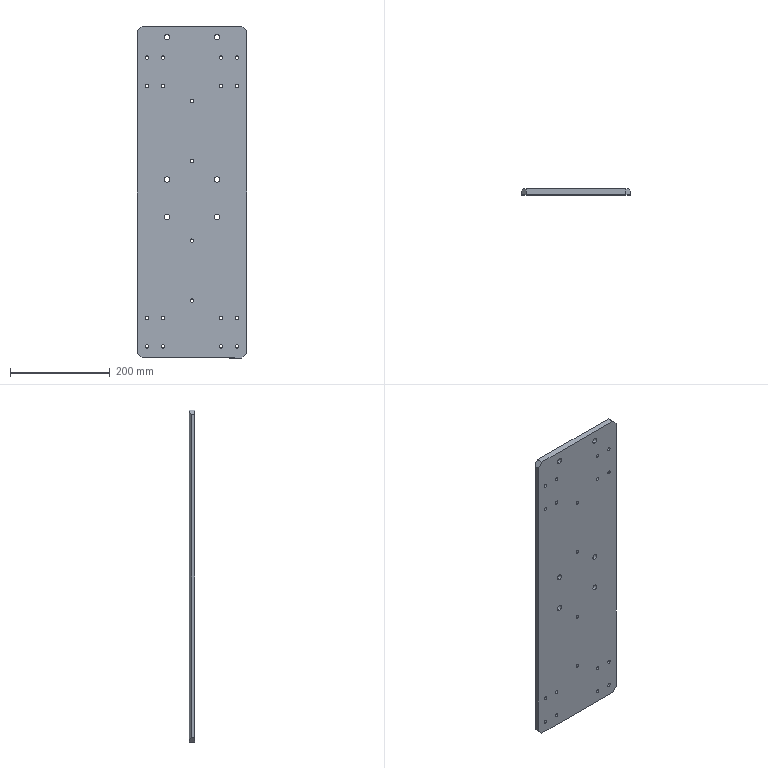Part | STEP file | PLACA BASE POLIPASTO | 1 solid | 64 faces | box 220 x 12 x 665 mm | volume 1721433 mm3 | cylinder 52 | plane 12 | commonest cylinder face diameters 6.8 x40 11 x12